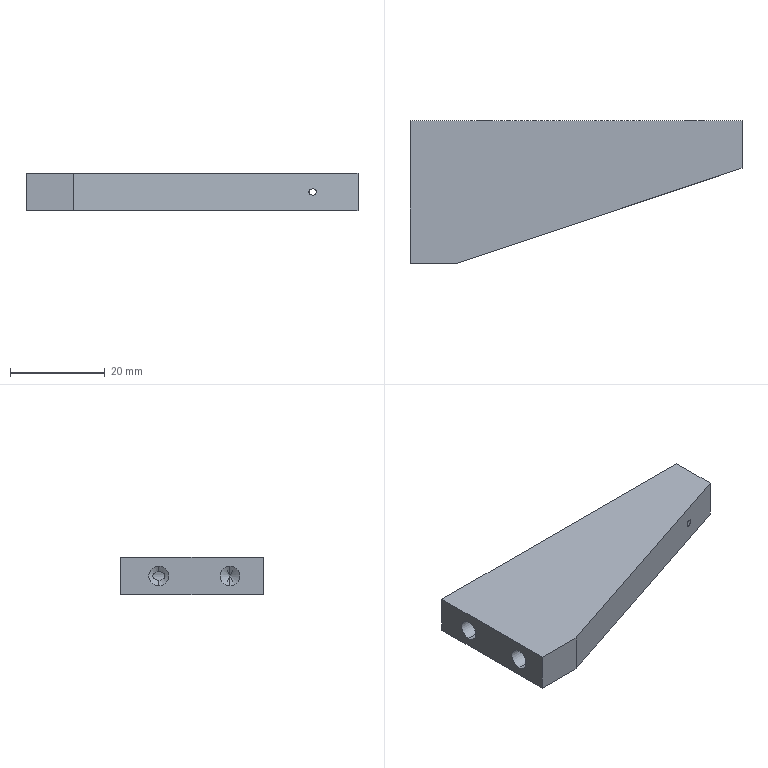Part | STEP file | FBDS-CS-016 | 1 solid | 23 faces | box 70 x 30 x 8 mm | volume 11291 mm3 | cylinder 8 | cone 8 | plane 7 | commonest cylinder face diameters 4.2 x8
STEP:
#1=CARTESIAN_POINT('',(12.4,-8.,1.9));
#2=VERTEX_POINT('',#1);
#3=CARTESIAN_POINT('',(12.4,-8.,6.1));
#4=VERTEX_POINT('',#3);
#5=CARTESIAN_POINT('',(12.4,-8.,4.));
#6=DIRECTION('',(-1.,0.,0.));
#7=DIRECTION('',(0.,0.,1.));
#8=AXIS2_PLACEMENT_3D('',#5,#6,#7);
#9=CIRCLE('',#8,2.1);
#10=EDGE_CURVE('',#2,#4,#9,.T.);
#11=ORIENTED_EDGE('',*,*,#10,.F.);
#12=CARTESIAN_POINT('',(0.,-8.,1.9));
#13=VERTEX_POINT('',#12);
#14=CARTESIAN_POINT('',(0.,-8.,1.9));
#15=DIRECTION('',(-1.,0.,0.));
#16=VECTOR('',#15,1000.);
#17=LINE('',#14,#16);
#18=EDGE_CURVE('',#2,#13,#17,.T.);
#19=ORIENTED_EDGE('',*,*,#18,.T.);
#20=CARTESIAN_POINT('',(0.,-8.,6.1));
#21=VERTEX_POINT('',#20);
#22=CARTESIAN_POINT('',(0.,-8.,4.));
#23=DIRECTION('',(-1.,0.,0.));
#24=DIRECTION('',(0.,0.,1.));
#25=AXIS2_PLACEMENT_3D('',#22,#23,#24);
#26=CIRCLE('',#25,2.1);
#27=EDGE_CURVE('',#13,#21,#26,.T.);
#28=ORIENTED_EDGE('',*,*,#27,.T.);
#29=CARTESIAN_POINT('',(0.,-8.,6.1));
#30=DIRECTION('',(-1.,0.,0.));
#31=VECTOR('',#30,1000.);
#32=LINE('',#29,#31);
#33=EDGE_CURVE('',#4,#21,#32,.T.);
#34=ORIENTED_EDGE('',*,*,#33,.F.);
#35=EDGE_LOOP('',(#11,#19,#28,#34));
#36=FACE_OUTER_BOUND('',#35,.T.);
#37=CARTESIAN_POINT('',(0.,-8.,4.));
#38=DIRECTION('',(-1.,0.,0.));
#39=DIRECTION('',(0.,0.,1.));
#40=AXIS2_PLACEMENT_3D('',#37,#38,#39);
#41=CYLINDRICAL_SURFACE('',#40,2.1);
#42=ADVANCED_FACE('',(#36),#41,.F.);
#43=CARTESIAN_POINT('',(13.111,-8.,3.083));
#44=VERTEX_POINT('',#43);
#45=CARTESIAN_POINT('',(13.111,-8.,4.917));
#46=VERTEX_POINT('',#45);
#47=CARTESIAN_POINT('',(13.111,-8.,3.083));
#48=CARTESIAN_POINT('',(13.111,-8.144,3.083));
#49=CARTESIAN_POINT('',(13.101,-8.29,3.102));
#50=CARTESIAN_POINT('',(13.068,-8.565,3.177));
#51=CARTESIAN_POINT('',(13.044,-8.699,3.233));
#52=CARTESIAN_POINT('',(12.991,-8.94,3.383));
#53=CARTESIAN_POINT('',(12.962,-9.05,3.478));
#54=CARTESIAN_POINT('',(12.916,-9.214,3.712));
#55=CARTESIAN_POINT('',(12.9,-9.268,3.855));
#56=CARTESIAN_POINT('',(12.9,-9.268,4.072));
#57=CARTESIAN_POINT('',(12.904,-9.255,4.145));
#58=CARTESIAN_POINT('',(12.918,-9.208,4.282));
#59=CARTESIAN_POINT('',(12.928,-9.173,4.346));
#60=CARTESIAN_POINT('',(12.962,-9.05,4.521));
#61=CARTESIAN_POINT('',(12.991,-8.94,4.617));
#62=CARTESIAN_POINT('',(13.07,-8.579,4.842));
#63=CARTESIAN_POINT('',(13.111,-8.287,4.917));
#64=CARTESIAN_POINT('',(13.111,-8.,4.917));
#65=B_SPLINE_CURVE_WITH_KNOTS('',3,(#47,#48,#49,#50,#51,#52,#53,#54,#55,#56,#57,#58,#59,#60,#61,#62,#63,#64),.UNSPECIFIED.,.F.,.F.,(4,2,2,2,2,2,2,2,4),(0.005551,0.005986,0.00642,0.006854,0.007288,0.007506,0.007723,0.008157,0.009026),.UNSPECIFIED.);
#66=EDGE_CURVE('',#44,#46,#65,.T.);
#67=ORIENTED_EDGE('',*,*,#66,.F.);
#68=CARTESIAN_POINT('',(12.4,-8.,1.9));
#69=DIRECTION('',(-0.515,0.,-0.8572));
#70=VECTOR('',#69,1000.);
#71=LINE('',#68,#70);
#72=EDGE_CURVE('',#44,#2,#71,.T.);
#73=ORIENTED_EDGE('',*,*,#72,.T.);
#74=ORIENTED_EDGE('',*,*,#10,.T.);
#75=CARTESIAN_POINT('',(12.4,-8.,6.1));
#76=DIRECTION('',(-0.515,0.,0.8572));
#77=VECTOR('',#76,1000.);
#78=LINE('',#75,#77);
#79=EDGE_CURVE('',#46,#4,#78,.T.);
#80=ORIENTED_EDGE('',*,*,#79,.F.);
#81=EDGE_LOOP('',(#67,#73,#74,#80));
#82=FACE_OUTER_BOUND('',#81,.T.);
#83=CARTESIAN_POINT('',(12.4,-8.,4.));
#84=DIRECTION('',(-1.,0.,0.));
#85=DIRECTION('',(0.,0.,1.));
#86=AXIS2_PLACEMENT_3D('',#83,#84,#85);
#87=CONICAL_SURFACE('',#86,2.1,1.03);
#88=ADVANCED_FACE('',(#82),#87,.F.);
#89=CARTESIAN_POINT('',(12.4,-23.,1.9));
#90=VERTEX_POINT('',#89);
#91=CARTESIAN_POINT('',(12.4,-23.,6.1));
#92=VERTEX_POINT('',#91);
#93=CARTESIAN_POINT('',(12.4,-23.,4.));
#94=DIRECTION('',(-1.,0.,0.));
#95=DIRECTION('',(0.,0.,1.));
#96=AXIS2_PLACEMENT_3D('',#93,#94,#95);
#97=CIRCLE('',#96,2.1);
#98=EDGE_CURVE('',#90,#92,#97,.T.);
#99=ORIENTED_EDGE('',*,*,#98,.F.);
#100=CARTESIAN_POINT('',(0.,-23.,1.9));
#101=VERTEX_POINT('',#100);
#102=CARTESIAN_POINT('',(0.,-23.,1.9));
#103=DIRECTION('',(-1.,0.,0.));
#104=VECTOR('',#103,1000.);
#105=LINE('',#102,#104);
#106=EDGE_CURVE('',#90,#101,#105,.T.);
#107=ORIENTED_EDGE('',*,*,#106,.T.);
#108=CARTESIAN_POINT('',(0.,-23.,6.1));
#109=VERTEX_POINT('',#108);
#110=CARTESIAN_POINT('',(0.,-23.,4.));
#111=DIRECTION('',(-1.,0.,0.));
#112=DIRECTION('',(0.,0.,1.));
#113=AXIS2_PLACEMENT_3D('',#110,#111,#112);
#114=CIRCLE('',#113,2.1);
#115=EDGE_CURVE('',#101,#109,#114,.T.);
#116=ORIENTED_EDGE('',*,*,#115,.T.);
#117=CARTESIAN_POINT('',(0.,-23.,6.1));
#118=DIRECTION('',(-1.,0.,0.));
#119=VECTOR('',#118,1000.);
#120=LINE('',#117,#119);
#121=EDGE_CURVE('',#92,#109,#120,.T.);
#122=ORIENTED_EDGE('',*,*,#121,.F.);
#123=EDGE_LOOP('',(#99,#107,#116,#122));
#124=FACE_OUTER_BOUND('',#123,.T.);
#125=CARTESIAN_POINT('',(0.,-23.,4.));
#126=DIRECTION('',(-1.,0.,0.));
#127=DIRECTION('',(0.,0.,1.));
#128=AXIS2_PLACEMENT_3D('',#125,#126,#127);
#129=CYLINDRICAL_SURFACE('',#128,2.1);
#130=ADVANCED_FACE('',(#124),#129,.F.);
#131=CARTESIAN_POINT('',(13.662,-23.,4.));
#132=VERTEX_POINT('',#131);
#133=CARTESIAN_POINT('',(12.4,-23.,6.1));
#134=DIRECTION('',(-0.515,0.,0.8572));
#135=VECTOR('',#134,1000.);
#136=LINE('',#133,#135);
#137=EDGE_CURVE('',#132,#92,#136,.T.);
#138=ORIENTED_EDGE('',*,*,#137,.F.);
#139=CARTESIAN_POINT('',(12.4,-23.,1.9));
#140=DIRECTION('',(-0.515,0.,-0.8572));
#141=VECTOR('',#140,1000.);
#142=LINE('',#139,#141);
#143=EDGE_CURVE('',#132,#90,#142,.T.);
#144=ORIENTED_EDGE('',*,*,#143,.T.);
#145=ORIENTED_EDGE('',*,*,#98,.T.);
#146=EDGE_LOOP('',(#138,#144,#145));
#147=FACE_OUTER_BOUND('',#146,.T.);
#148=CARTESIAN_POINT('',(12.4,-23.,4.));
#149=DIRECTION('',(-1.,0.,0.));
#150=DIRECTION('',(0.,0.,1.));
#151=AXIS2_PLACEMENT_3D('',#148,#149,#150);
#152=CONICAL_SURFACE('',#151,2.1,1.03);
#153=ADVANCED_FACE('',(#147),#152,.F.);
#154=CARTESIAN_POINT('',(13.111,-8.,4.917));
#155=CARTESIAN_POINT('',(13.111,-7.856,4.917));
#156=CARTESIAN_POINT('',(13.101,-7.71,4.898));
#157=CARTESIAN_POINT('',(13.068,-7.435,4.823));
#158=CARTESIAN_POINT('',(13.044,-7.301,4.767));
#159=CARTESIAN_POINT('',(12.991,-7.06,4.617));
#160=CARTESIAN_POINT('',(12.962,-6.95,4.522));
#161=CARTESIAN_POINT('',(12.928,-6.827,4.347));
#162=CARTESIAN_POINT('',(12.918,-6.792,4.282));
#163=CARTESIAN_POINT('',(12.904,-6.745,4.146));
#164=CARTESIAN_POINT('',(12.9,-6.732,4.073));
#165=CARTESIAN_POINT('',(12.9,-6.732,3.856));
#166=CARTESIAN_POINT('',(12.916,-6.786,3.712));
#167=CARTESIAN_POINT('',(12.962,-6.95,3.479));
#168=CARTESIAN_POINT('',(12.991,-7.06,3.383));
#169=CARTESIAN_POINT('',(13.07,-7.421,3.158));
#170=CARTESIAN_POINT('',(13.111,-7.713,3.083));
#171=CARTESIAN_POINT('',(13.111,-8.,3.083));
#172=B_SPLINE_CURVE_WITH_KNOTS('',3,(#154,#155,#156,#157,#158,#159,#160,#161,#162,#163,#164,#165,#166,#167,#168,#169,#170,#171),.UNSPECIFIED.,.F.,.F.,(4,2,2,2,2,2,2,2,4),(0.002077,0.002511,0.002945,0.00338,0.003597,0.003814,0.004248,0.004683,0.005551),.UNSPECIFIED.);
#173=EDGE_CURVE('',#46,#44,#172,.T.);
#174=ORIENTED_EDGE('',*,*,#173,.T.);
#175=ORIENTED_EDGE('',*,*,#66,.T.);
#176=EDGE_LOOP('',(#174,#175));
#177=FACE_BOUND('',#176,.T.);
#178=CARTESIAN_POINT('',(15.,-12.4,1.9));
#179=VERTEX_POINT('',#178);
#180=CARTESIAN_POINT('',(15.,-12.4,6.1));
#181=VERTEX_POINT('',#180);
#182=CARTESIAN_POINT('',(15.,-12.4,4.));
#183=DIRECTION('',(0.,1.,0.));
#184=DIRECTION('',(0.,0.,1.));
#185=AXIS2_PLACEMENT_3D('',#182,#183,#184);
#186=CIRCLE('',#185,2.1);
#187=EDGE_CURVE('',#179,#181,#186,.T.);
#188=ORIENTED_EDGE('',*,*,#187,.F.);
#189=CARTESIAN_POINT('',(15.,0.,1.9));
#190=VERTEX_POINT('',#189);
#191=CARTESIAN_POINT('',(15.,0.,1.9));
#192=DIRECTION('',(0.,1.,0.));
#193=VECTOR('',#192,1000.);
#194=LINE('',#191,#193);
#195=EDGE_CURVE('',#179,#190,#194,.T.);
#196=ORIENTED_EDGE('',*,*,#195,.T.);
#197=CARTESIAN_POINT('',(15.,0.,6.1));
#198=VERTEX_POINT('',#197);
#199=CARTESIAN_POINT('',(15.,0.,4.));
#200=DIRECTION('',(0.,1.,0.));
#201=DIRECTION('',(0.,0.,1.));
#202=AXIS2_PLACEMENT_3D('',#199,#200,#201);
#203=CIRCLE('',#202,2.1);
#204=EDGE_CURVE('',#190,#198,#203,.T.);
#205=ORIENTED_EDGE('',*,*,#204,.T.);
#206=CARTESIAN_POINT('',(15.,0.,6.1));
#207=DIRECTION('',(0.,1.,0.));
#208=VECTOR('',#207,1000.);
#209=LINE('',#206,#208);
#210=EDGE_CURVE('',#181,#198,#209,.T.);
#211=ORIENTED_EDGE('',*,*,#210,.F.);
#212=EDGE_LOOP('',(#188,#196,#205,#211));
#213=FACE_OUTER_BOUND('',#212,.T.);
#214=CARTESIAN_POINT('',(15.,0.,4.));
#215=DIRECTION('',(0.,1.,0.));
#216=DIRECTION('',(0.,0.,1.));
#217=AXIS2_PLACEMENT_3D('',#214,#215,#216);
#218=CYLINDRICAL_SURFACE('',#217,2.1);
#219=ADVANCED_FACE('',(#177,#213),#218,.F.);
#220=CARTESIAN_POINT('',(15.,-13.662,4.));
#221=VERTEX_POINT('',#220);
#222=CARTESIAN_POINT('',(15.,-12.4,6.1));
#223=DIRECTION('',(0.,0.515,0.8572));
#224=VECTOR('',#223,1000.);
#225=LINE('',#222,#224);
#226=EDGE_CURVE('',#221,#181,#225,.T.);
#227=ORIENTED_EDGE('',*,*,#226,.F.);
#228=CARTESIAN_POINT('',(15.,-12.4,1.9));
#229=DIRECTION('',(0.,0.515,-0.8572));
#230=VECTOR('',#229,1000.);
#231=LINE('',#228,#230);
#232=EDGE_CURVE('',#221,#179,#231,.T.);
#233=ORIENTED_EDGE('',*,*,#232,.T.);
#234=ORIENTED_EDGE('',*,*,#187,.T.);
#235=EDGE_LOOP('',(#227,#233,#234));
#236=FACE_OUTER_BOUND('',#235,.T.);
#237=CARTESIAN_POINT('',(15.,-12.4,4.));
#238=DIRECTION('',(0.,1.,0.));
#239=DIRECTION('',(0.,0.,1.));
#240=AXIS2_PLACEMENT_3D('',#237,#238,#239);
#241=CONICAL_SURFACE('',#240,2.1,1.03);
#242=ADVANCED_FACE('',(#236),#241,.F.);
#243=CARTESIAN_POINT('',(60.,-12.4,1.9));
#244=VERTEX_POINT('',#243);
#245=CARTESIAN_POINT('',(60.,-12.4,6.1));
#246=VERTEX_POINT('',#245);
#247=CARTESIAN_POINT('',(60.,-12.4,4.));
#248=DIRECTION('',(0.,1.,0.));
#249=DIRECTION('',(0.,0.,1.));
#250=AXIS2_PLACEMENT_3D('',#247,#248,#249);
#251=CIRCLE('',#250,2.1);
#252=EDGE_CURVE('',#244,#246,#251,.T.);
#253=ORIENTED_EDGE('',*,*,#252,.F.);
#254=CARTESIAN_POINT('',(60.,0.,1.9));
#255=VERTEX_POINT('',#254);
#256=CARTESIAN_POINT('',(60.,0.,1.9));
#257=DIRECTION('',(0.,1.,0.));
#258=VECTOR('',#257,1000.);
#259=LINE('',#256,#258);
#260=EDGE_CURVE('',#244,#255,#259,.T.);
#261=ORIENTED_EDGE('',*,*,#260,.T.);
#262=CARTESIAN_POINT('',(60.,0.,6.1));
#263=VERTEX_POINT('',#262);
#264=CARTESIAN_POINT('',(60.,0.,4.));
#265=DIRECTION('',(0.,1.,0.));
#266=DIRECTION('',(0.,0.,1.));
#267=AXIS2_PLACEMENT_3D('',#264,#265,#266);
#268=CIRCLE('',#267,2.1);
#269=EDGE_CURVE('',#255,#263,#268,.T.);
#270=ORIENTED_EDGE('',*,*,#269,.T.);
#271=CARTESIAN_POINT('',(60.,0.,6.1));
#272=DIRECTION('',(0.,1.,0.));
#273=VECTOR('',#272,1000.);
#274=LINE('',#271,#273);
#275=EDGE_CURVE('',#246,#263,#274,.T.);
#276=ORIENTED_EDGE('',*,*,#275,.F.);
#277=EDGE_LOOP('',(#253,#261,#270,#276));
#278=FACE_OUTER_BOUND('',#277,.T.);
#279=CARTESIAN_POINT('',(60.,0.,4.));
#280=DIRECTION('',(0.,1.,0.));
#281=DIRECTION('',(0.,0.,1.));
#282=AXIS2_PLACEMENT_3D('',#279,#280,#281);
#283=CYLINDRICAL_SURFACE('',#282,2.1);
#284=ADVANCED_FACE('',(#278),#283,.F.);
#285=CARTESIAN_POINT('',(60.,-13.333,3.453));
#286=VERTEX_POINT('',#285);
#287=CARTESIAN_POINT('',(60.,-13.333,4.547));
#288=VERTEX_POINT('',#287);
#289=CARTESIAN_POINT('',(60.,-13.333,3.453));
#290=CARTESIAN_POINT('',(59.482,-13.506,3.741));
#291=CARTESIAN_POINT('',(59.482,-13.506,4.259));
#292=CARTESIAN_POINT('',(60.,-13.333,4.547));
#293=(BOUNDED_CURVE()B_SPLINE_CURVE(3,(#289,#290,#291,#292),.UNSPECIFIED.,.F.,.F.)B_SPLINE_CURVE_WITH_KNOTS((4,4),(2.159,4.124),.UNSPECIFIED.)CURVE()GEOMETRIC_REPRESENTATION_ITEM()RATIONAL_B_SPLINE_CURVE((1.,0.7032,0.7032,1.))REPRESENTATION_ITEM(''));
#294=EDGE_CURVE('',#286,#288,#293,.T.);
#295=ORIENTED_EDGE('',*,*,#294,.F.);
#296=CARTESIAN_POINT('',(60.,-12.4,1.9));
#297=DIRECTION('',(0.,0.515,-0.8572));
#298=VECTOR('',#297,1000.);
#299=LINE('',#296,#298);
#300=EDGE_CURVE('',#286,#244,#299,.T.);
#301=ORIENTED_EDGE('',*,*,#300,.T.);
#302=ORIENTED_EDGE('',*,*,#252,.T.);
#303=CARTESIAN_POINT('',(60.,-12.4,6.1));
#304=DIRECTION('',(0.,0.515,0.8572));
#305=VECTOR('',#304,1000.);
#306=LINE('',#303,#305);
#307=EDGE_CURVE('',#288,#246,#306,.T.);
#308=ORIENTED_EDGE('',*,*,#307,.F.);
#309=EDGE_LOOP('',(#295,#301,#302,#308));
#310=FACE_OUTER_BOUND('',#309,.T.);
#311=CARTESIAN_POINT('',(60.,-12.4,4.));
#312=DIRECTION('',(0.,1.,0.));
#313=DIRECTION('',(0.,0.,1.));
#314=AXIS2_PLACEMENT_3D('',#311,#312,#313);
#315=CONICAL_SURFACE('',#314,2.1,1.03);
#316=ADVANCED_FACE('',(#310),#315,.F.);
#317=CARTESIAN_POINT('',(0.,-8.,4.));
#318=DIRECTION('',(-1.,0.,0.));
#319=DIRECTION('',(0.,0.,1.));
#320=AXIS2_PLACEMENT_3D('',#317,#318,#319);
#321=CIRCLE('',#320,2.1);
#322=EDGE_CURVE('',#21,#13,#321,.T.);
#323=ORIENTED_EDGE('',*,*,#322,.F.);
#324=ORIENTED_EDGE('',*,*,#27,.F.);
#325=EDGE_LOOP('',(#323,#324));
#326=FACE_BOUND('',#325,.T.);
#327=CARTESIAN_POINT('',(0.,-23.,4.));
#328=DIRECTION('',(-1.,0.,0.));
#329=DIRECTION('',(0.,0.,1.));
#330=AXIS2_PLACEMENT_3D('',#327,#328,#329);
#331=CIRCLE('',#330,2.1);
#332=EDGE_CURVE('',#109,#101,#331,.T.);
#333=ORIENTED_EDGE('',*,*,#332,.F.);
#334=ORIENTED_EDGE('',*,*,#115,.F.);
#335=EDGE_LOOP('',(#333,#334));
#336=FACE_BOUND('',#335,.T.);
#337=CARTESIAN_POINT('',(0.,0.,0.));
#338=VERTEX_POINT('',#337);
#339=CARTESIAN_POINT('',(0.,-30.,0.));
#340=VERTEX_POINT('',#339);
#341=CARTESIAN_POINT('',(0.,-30.,0.));
#342=DIRECTION('',(0.,-1.,0.));
#343=VECTOR('',#342,1000.);
#344=LINE('',#341,#343);
#345=EDGE_CURVE('',#338,#340,#344,.T.);
#346=ORIENTED_EDGE('',*,*,#345,.T.);
#347=CARTESIAN_POINT('',(0.,-30.,8.));
#348=VERTEX_POINT('',#347);
#349=CARTESIAN_POINT('',(0.,-30.,8.));
#350=DIRECTION('',(0.,0.,-1.));
#351=VECTOR('',#350,1000.);
#352=LINE('',#349,#351);
#353=EDGE_CURVE('',#348,#340,#352,.T.);
#354=ORIENTED_EDGE('',*,*,#353,.F.);
#355=CARTESIAN_POINT('',(0.,0.,8.));
#356=VERTEX_POINT('',#355);
#357=CARTESIAN_POINT('',(0.,-30.,8.));
#358=DIRECTION('',(0.,-1.,0.));
#359=VECTOR('',#358,1000.);
#360=LINE('',#357,#359);
#361=EDGE_CURVE('',#356,#348,#360,.T.);
#362=ORIENTED_EDGE('',*,*,#361,.F.);
#363=CARTESIAN_POINT('',(0.,0.,8.));
#364=DIRECTION('',(0.,0.,-1.));
#365=VECTOR('',#364,1000.);
#366=LINE('',#363,#365);
#367=EDGE_CURVE('',#356,#338,#366,.T.);
#368=ORIENTED_EDGE('',*,*,#367,.T.);
#369=EDGE_LOOP('',(#346,#354,#362,#368));
#370=FACE_OUTER_BOUND('',#369,.T.);
#371=CARTESIAN_POINT('',(0.,-30.,8.));
#372=DIRECTION('',(1.,0.,0.));
#373=DIRECTION('',(0.,0.,-1.));
#374=AXIS2_PLACEMENT_3D('',#371,#372,#373);
#375=PLANE('',#374);
#376=ADVANCED_FACE('',(#326,#336,#370),#375,.F.);
#377=CARTESIAN_POINT('',(10.,-30.,0.));
#378=VERTEX_POINT('',#377);
#379=CARTESIAN_POINT('',(10.,-30.,0.));
#380=DIRECTION('',(1.,0.,0.));
#381=VECTOR('',#380,1000.);
#382=LINE('',#379,#381);
#383=EDGE_CURVE('',#340,#378,#382,.T.);
#384=ORIENTED_EDGE('',*,*,#383,.T.);
#385=CARTESIAN_POINT('',(10.,-30.,8.));
#386=VERTEX_POINT('',#385);
#387=CARTESIAN_POINT('',(10.,-30.,8.));
#388=DIRECTION('',(0.,0.,-1.));
#389=VECTOR('',#388,1000.);
#390=LINE('',#387,#389);
#391=EDGE_CURVE('',#386,#378,#390,.T.);
#392=ORIENTED_EDGE('',*,*,#391,.F.);
#393=CARTESIAN_POINT('',(10.,-30.,8.));
#394=DIRECTION('',(1.,0.,0.));
#395=VECTOR('',#394,1000.);
#396=LINE('',#393,#395);
#397=EDGE_CURVE('',#348,#386,#396,.T.);
#398=ORIENTED_EDGE('',*,*,#397,.F.);
#399=ORIENTED_EDGE('',*,*,#353,.T.);
#400=EDGE_LOOP('',(#384,#392,#398,#399));
#401=FACE_OUTER_BOUND('',#400,.T.);
#402=CARTESIAN_POINT('',(10.,-30.,8.));
#403=DIRECTION('',(0.,1.,0.));
#404=DIRECTION('',(0.,0.,1.));
#405=AXIS2_PLACEMENT_3D('',#402,#403,#404);
#406=PLANE('',#405);
#407=ADVANCED_FACE('',(#401),#406,.F.);
#408=CARTESIAN_POINT('',(60.,-13.333,4.547));
#409=CARTESIAN_POINT('',(60.596,-13.135,4.877));
#410=CARTESIAN_POINT('',(61.228,-12.924,4.596));
#411=CARTESIAN_POINT('',(61.228,-12.924,4.));
#412=CARTESIAN_POINT('',(61.228,-12.924,3.404));
#413=CARTESIAN_POINT('',(60.596,-13.135,3.123));
#414=CARTESIAN_POINT('',(60.,-13.333,3.453));
#415=(BOUNDED_CURVE()B_SPLINE_CURVE(3,(#408,#409,#410,#411,#412,#413,#414),.UNSPECIFIED.,.F.,.F.)B_SPLINE_CURVE_WITH_KNOTS((4,3,4),(4.124,6.283,8.442),.UNSPECIFIED.)CURVE()GEOMETRIC_REPRESENTATION_ITEM()RATIONAL_B_SPLINE_CURVE((1.,0.6479,0.6479,1.,0.6479,0.6479,1.))REPRESENTATION_ITEM(''));
#416=EDGE_CURVE('',#288,#286,#415,.T.);
#417=ORIENTED_EDGE('',*,*,#416,.T.);
#418=ORIENTED_EDGE('',*,*,#294,.T.);
#419=EDGE_LOOP('',(#417,#418));
#420=FACE_BOUND('',#419,.T.);
#421=CARTESIAN_POINT('',(70.,-10.,0.));
#422=VERTEX_POINT('',#421);
#423=CARTESIAN_POINT('',(70.,-10.,0.));
#424=DIRECTION('',(0.9487,0.3162,0.));
#425=VECTOR('',#424,1000.);
#426=LINE('',#423,#425);
#427=EDGE_CURVE('',#378,#422,#426,.T.);
#428=ORIENTED_EDGE('',*,*,#427,.T.);
#429=CARTESIAN_POINT('',(70.,-10.,8.));
#430=VERTEX_POINT('',#429);
#431=CARTESIAN_POINT('',(70.,-10.,8.));
#432=DIRECTION('',(0.,0.,-1.));
#433=VECTOR('',#432,1000.);
#434=LINE('',#431,#433);
#435=EDGE_CURVE('',#430,#422,#434,.T.);
#436=ORIENTED_EDGE('',*,*,#435,.F.);
#437=CARTESIAN_POINT('',(70.,-10.,8.));
#438=DIRECTION('',(0.9487,0.3162,0.));
#439=VECTOR('',#438,1000.);
#440=LINE('',#437,#439);
#441=EDGE_CURVE('',#386,#430,#440,.T.);
#442=ORIENTED_EDGE('',*,*,#441,.F.);
#443=ORIENTED_EDGE('',*,*,#391,.T.);
#444=EDGE_LOOP('',(#428,#436,#442,#443));
#445=FACE_OUTER_BOUND('',#444,.T.);
#446=CARTESIAN_POINT('',(70.,-10.,8.));
#447=DIRECTION('',(-0.3162,0.9487,0.));
#448=DIRECTION('',(-0.9487,-0.3162,0.));
#449=AXIS2_PLACEMENT_3D('',#446,#447,#448);
#450=PLANE('',#449);
#451=ADVANCED_FACE('',(#420,#445),#450,.F.);
#452=CARTESIAN_POINT('',(70.,0.,0.));
#453=VERTEX_POINT('',#452);
#454=CARTESIAN_POINT('',(70.,0.,0.));
#455=DIRECTION('',(0.,1.,0.));
#456=VECTOR('',#455,1000.);
#457=LINE('',#454,#456);
#458=EDGE_CURVE('',#422,#453,#457,.T.);
#459=ORIENTED_EDGE('',*,*,#458,.T.);
#460=CARTESIAN_POINT('',(70.,0.,8.));
#461=VERTEX_POINT('',#460);
#462=CARTESIAN_POINT('',(70.,0.,8.));
#463=DIRECTION('',(0.,0.,-1.));
#464=VECTOR('',#463,1000.);
#465=LINE('',#462,#464);
#466=EDGE_CURVE('',#461,#453,#465,.T.);
#467=ORIENTED_EDGE('',*,*,#466,.F.);
#468=CARTESIAN_POINT('',(70.,0.,8.));
#469=DIRECTION('',(0.,1.,0.));
#470=VECTOR('',#469,1000.);
#471=LINE('',#468,#470);
#472=EDGE_CURVE('',#430,#461,#471,.T.);
#473=ORIENTED_EDGE('',*,*,#472,.F.);
#474=ORIENTED_EDGE('',*,*,#435,.T.);
#475=EDGE_LOOP('',(#459,#467,#473,#474));
#476=FACE_OUTER_BOUND('',#475,.T.);
#477=CARTESIAN_POINT('',(70.,0.,8.));
#478=DIRECTION('',(-1.,0.,0.));
#479=DIRECTION('',(0.,0.,1.));
#480=AXIS2_PLACEMENT_3D('',#477,#478,#479);
#481=PLANE('',#480);
#482=ADVANCED_FACE('',(#476),#481,.F.);
#483=CARTESIAN_POINT('',(15.,0.,4.));
#484=DIRECTION('',(0.,1.,0.));
#485=DIRECTION('',(0.,0.,1.));
#486=AXIS2_PLACEMENT_3D('',#483,#484,#485);
#487=CIRCLE('',#486,2.1);
#488=EDGE_CURVE('',#198,#190,#487,.T.);
#489=ORIENTED_EDGE('',*,*,#488,.F.);
#490=ORIENTED_EDGE('',*,*,#204,.F.);
#491=EDGE_LOOP('',(#489,#490));
#492=FACE_BOUND('',#491,.T.);
#493=CARTESIAN_POINT('',(60.,0.,4.));
#494=DIRECTION('',(0.,1.,0.));
#495=DIRECTION('',(0.,0.,1.));
#496=AXIS2_PLACEMENT_3D('',#493,#494,#495);
#497=CIRCLE('',#496,2.1);
#498=EDGE_CURVE('',#263,#255,#497,.T.);
#499=ORIENTED_EDGE('',*,*,#498,.F.);
#500=ORIENTED_EDGE('',*,*,#269,.F.);
#501=EDGE_LOOP('',(#499,#500));
#502=FACE_BOUND('',#501,.T.);
#503=CARTESIAN_POINT('',(0.,0.,0.));
#504=DIRECTION('',(-1.,0.,0.));
#505=VECTOR('',#504,1000.);
#506=LINE('',#503,#505);
#507=EDGE_CURVE('',#453,#338,#506,.T.);
#508=ORIENTED_EDGE('',*,*,#507,.T.);
#509=ORIENTED_EDGE('',*,*,#367,.F.);
#510=CARTESIAN_POINT('',(0.,0.,8.));
#511=DIRECTION('',(-1.,0.,0.));
#512=VECTOR('',#511,1000.);
#513=LINE('',#510,#512);
#514=EDGE_CURVE('',#461,#356,#513,.T.);
#515=ORIENTED_EDGE('',*,*,#514,.F.);
#516=ORIENTED_EDGE('',*,*,#466,.T.);
#517=EDGE_LOOP('',(#508,#509,#515,#516));
#518=FACE_OUTER_BOUND('',#517,.T.);
#519=CARTESIAN_POINT('',(0.,0.,8.));
#520=DIRECTION('',(0.,-1.,0.));
#521=DIRECTION('',(0.,0.,-1.));
#522=AXIS2_PLACEMENT_3D('',#519,#520,#521);
#523=PLANE('',#522);
#524=ADVANCED_FACE('',(#492,#502,#518),#523,.F.);
#525=ORIENTED_EDGE('',*,*,#361,.T.);
#526=ORIENTED_EDGE('',*,*,#397,.T.);
#527=ORIENTED_EDGE('',*,*,#441,.T.);
#528=ORIENTED_EDGE('',*,*,#472,.T.);
#529=ORIENTED_EDGE('',*,*,#514,.T.);
#530=EDGE_LOOP('',(#525,#526,#527,#528,#529));
#531=FACE_OUTER_BOUND('',#530,.T.);
#532=CARTESIAN_POINT('',(0.,0.,8.));
#533=DIRECTION('',(0.,0.,-1.));
#534=DIRECTION('',(-1.,0.,0.));
#535=AXIS2_PLACEMENT_3D('',#532,#533,#534);
#536=PLANE('',#535);
#537=ADVANCED_FACE('',(#531),#536,.F.);
#538=ORIENTED_EDGE('',*,*,#345,.F.);
#539=ORIENTED_EDGE('',*,*,#507,.F.);
#540=ORIENTED_EDGE('',*,*,#458,.F.);
#541=ORIENTED_EDGE('',*,*,#427,.F.);
#542=ORIENTED_EDGE('',*,*,#383,.F.);
#543=EDGE_LOOP('',(#538,#539,#540,#541,#542));
#544=FACE_OUTER_BOUND('',#543,.T.);
#545=CARTESIAN_POINT('',(0.,0.,0.));
#546=DIRECTION('',(0.,0.,-1.));
#547=DIRECTION('',(-1.,0.,0.));
#548=AXIS2_PLACEMENT_3D('',#545,#546,#547);
#549=PLANE('',#548);
#550=ADVANCED_FACE('',(#544),#549,.T.);
#551=ORIENTED_EDGE('',*,*,#300,.F.);
#552=ORIENTED_EDGE('',*,*,#416,.F.);
#553=ORIENTED_EDGE('',*,*,#307,.T.);
#554=CARTESIAN_POINT('',(60.,-12.4,4.));
#555=DIRECTION('',(0.,1.,0.));
#556=DIRECTION('',(0.,0.,1.));
#557=AXIS2_PLACEMENT_3D('',#554,#555,#556);
#558=CIRCLE('',#557,2.1);
#559=EDGE_CURVE('',#246,#244,#558,.T.);
#560=ORIENTED_EDGE('',*,*,#559,.T.);
#561=EDGE_LOOP('',(#551,#552,#553,#560));
#562=FACE_OUTER_BOUND('',#561,.T.);
#563=CARTESIAN_POINT('',(60.,-12.4,4.));
#564=DIRECTION('',(0.,1.,0.));
#565=DIRECTION('',(0.,0.,1.));
#566=AXIS2_PLACEMENT_3D('',#563,#564,#565);
#567=CONICAL_SURFACE('',#566,2.1,1.03);
#568=ADVANCED_FACE('',(#562),#567,.F.);
#569=ORIENTED_EDGE('',*,*,#260,.F.);
#570=ORIENTED_EDGE('',*,*,#559,.F.);
#571=ORIENTED_EDGE('',*,*,#275,.T.);
#572=ORIENTED_EDGE('',*,*,#498,.T.);
#573=EDGE_LOOP('',(#569,#570,#571,#572));
#574=FACE_OUTER_BOUND('',#573,.T.);
#575=CARTESIAN_POINT('',(60.,0.,4.));
#576=DIRECTION('',(0.,1.,0.));
#577=DIRECTION('',(0.,0.,1.));
#578=AXIS2_PLACEMENT_3D('',#575,#576,#577);
#579=CYLINDRICAL_SURFACE('',#578,2.1);
#580=ADVANCED_FACE('',(#574),#579,.F.);
#581=ORIENTED_EDGE('',*,*,#232,.F.);
#582=ORIENTED_EDGE('',*,*,#226,.T.);
#583=CARTESIAN_POINT('',(15.,-12.4,4.));
#584=DIRECTION('',(0.,1.,0.));
#585=DIRECTION('',(0.,0.,1.));
#586=AXIS2_PLACEMENT_3D('',#583,#584,#585);
#587=CIRCLE('',#586,2.1);
#588=EDGE_CURVE('',#181,#179,#587,.T.);
#589=ORIENTED_EDGE('',*,*,#588,.T.);
#590=EDGE_LOOP('',(#581,#582,#589));
#591=FACE_OUTER_BOUND('',#590,.T.);
#592=CARTESIAN_POINT('',(15.,-12.4,4.));
#593=DIRECTION('',(0.,1.,0.));
#594=DIRECTION('',(0.,0.,1.));
#595=AXIS2_PLACEMENT_3D('',#592,#593,#594);
#596=CONICAL_SURFACE('',#595,2.1,1.03);
#597=ADVANCED_FACE('',(#591),#596,.F.);
#598=ORIENTED_EDGE('',*,*,#195,.F.);
#599=ORIENTED_EDGE('',*,*,#588,.F.);
#600=ORIENTED_EDGE('',*,*,#210,.T.);
#601=ORIENTED_EDGE('',*,*,#488,.T.);
#602=EDGE_LOOP('',(#598,#599,#600,#601));
#603=FACE_OUTER_BOUND('',#602,.T.);
#604=CARTESIAN_POINT('',(15.,0.,4.));
#605=DIRECTION('',(0.,1.,0.));
#606=DIRECTION('',(0.,0.,1.));
#607=AXIS2_PLACEMENT_3D('',#604,#605,#606);
#608=CYLINDRICAL_SURFACE('',#607,2.1);
#609=ADVANCED_FACE('',(#603),#608,.F.);
#610=ORIENTED_EDGE('',*,*,#143,.F.);
#611=ORIENTED_EDGE('',*,*,#137,.T.);
#612=CARTESIAN_POINT('',(12.4,-23.,4.));
#613=DIRECTION('',(-1.,0.,0.));
#614=DIRECTION('',(0.,0.,1.));
#615=AXIS2_PLACEMENT_3D('',#612,#613,#614);
#616=CIRCLE('',#615,2.1);
#617=EDGE_CURVE('',#92,#90,#616,.T.);
#618=ORIENTED_EDGE('',*,*,#617,.T.);
#619=EDGE_LOOP('',(#610,#611,#618));
#620=FACE_OUTER_BOUND('',#619,.T.);
#621=CARTESIAN_POINT('',(12.4,-23.,4.));
#622=DIRECTION('',(-1.,0.,0.));
#623=DIRECTION('',(0.,0.,1.));
#624=AXIS2_PLACEMENT_3D('',#621,#622,#623);
#625=CONICAL_SURFACE('',#624,2.1,1.03);
#626=ADVANCED_FACE('',(#620),#625,.F.);
#627=ORIENTED_EDGE('',*,*,#106,.F.);
#628=ORIENTED_EDGE('',*,*,#617,.F.);
#629=ORIENTED_EDGE('',*,*,#121,.T.);
#630=ORIENTED_EDGE('',*,*,#332,.T.);
#631=EDGE_LOOP('',(#627,#628,#629,#630));
#632=FACE_OUTER_BOUND('',#631,.T.);
#633=CARTESIAN_POINT('',(0.,-23.,4.));
#634=DIRECTION('',(-1.,0.,0.));
#635=DIRECTION('',(0.,0.,1.));
#636=AXIS2_PLACEMENT_3D('',#633,#634,#635);
#637=CYLINDRICAL_SURFACE('',#636,2.1);
#638=ADVANCED_FACE('',(#632),#637,.F.);
#639=ORIENTED_EDGE('',*,*,#72,.F.);
#640=ORIENTED_EDGE('',*,*,#173,.F.);
#641=ORIENTED_EDGE('',*,*,#79,.T.);
#642=CARTESIAN_POINT('',(12.4,-8.,4.));
#643=DIRECTION('',(-1.,0.,0.));
#644=DIRECTION('',(0.,0.,1.));
#645=AXIS2_PLACEMENT_3D('',#642,#643,#644);
#646=CIRCLE('',#645,2.1);
#647=EDGE_CURVE('',#4,#2,#646,.T.);
#648=ORIENTED_EDGE('',*,*,#647,.T.);
#649=EDGE_LOOP('',(#639,#640,#641,#648));
#650=FACE_OUTER_BOUND('',#649,.T.);
#651=CARTESIAN_POINT('',(12.4,-8.,4.));
#652=DIRECTION('',(-1.,0.,0.));
#653=DIRECTION('',(0.,0.,1.));
#654=AXIS2_PLACEMENT_3D('',#651,#652,#653);
#655=CONICAL_SURFACE('',#654,2.1,1.03);
#656=ADVANCED_FACE('',(#650),#655,.F.);
#657=ORIENTED_EDGE('',*,*,#18,.F.);
#658=ORIENTED_EDGE('',*,*,#647,.F.);
#659=ORIENTED_EDGE('',*,*,#33,.T.);
#660=ORIENTED_EDGE('',*,*,#322,.T.);
#661=EDGE_LOOP('',(#657,#658,#659,#660));
#662=FACE_OUTER_BOUND('',#661,.T.);
#663=CARTESIAN_POINT('',(0.,-8.,4.));
#664=DIRECTION('',(-1.,0.,0.));
#665=DIRECTION('',(0.,0.,1.));
#666=AXIS2_PLACEMENT_3D('',#663,#664,#665);
#667=CYLINDRICAL_SURFACE('',#666,2.1);
#668=ADVANCED_FACE('',(#662),#667,.F.);
#669=CLOSED_SHELL('',(#42,#88,#130,#153,#219,#242,#284,#316,#376,#407,#451,#482,#524,#537,#550,#568,#580,#597,#609,#626,#638,#656,#668));
#670=MANIFOLD_SOLID_BREP('',#669);
#671=CARTESIAN_POINT('',(0.,0.,0.));
#672=DIRECTION('',(0.,0.,1.));
#673=DIRECTION('',(1.,0.,0.));
#674=AXIS2_PLACEMENT_3D('',#671,#672,#673);
#675=(LENGTH_UNIT()NAMED_UNIT(*)SI_UNIT(.MILLI.,.METRE.));
#676=UNCERTAINTY_MEASURE_WITH_UNIT(LENGTH_MEASURE(0.00001),#675,'','');
#677=(NAMED_UNIT(*)PLANE_ANGLE_UNIT()SI_UNIT($,.RADIAN.));
#678=(NAMED_UNIT(*)SI_UNIT($,.STERADIAN.)SOLID_ANGLE_UNIT());
#679=(GEOMETRIC_REPRESENTATION_CONTEXT(3)GLOBAL_UNCERTAINTY_ASSIGNED_CONTEXT((#676))GLOBAL_UNIT_ASSIGNED_CONTEXT((#675,#677,#678))REPRESENTATION_CONTEXT('',''));
#680=ADVANCED_BREP_SHAPE_REPRESENTATION('',(#670,#674),#679);